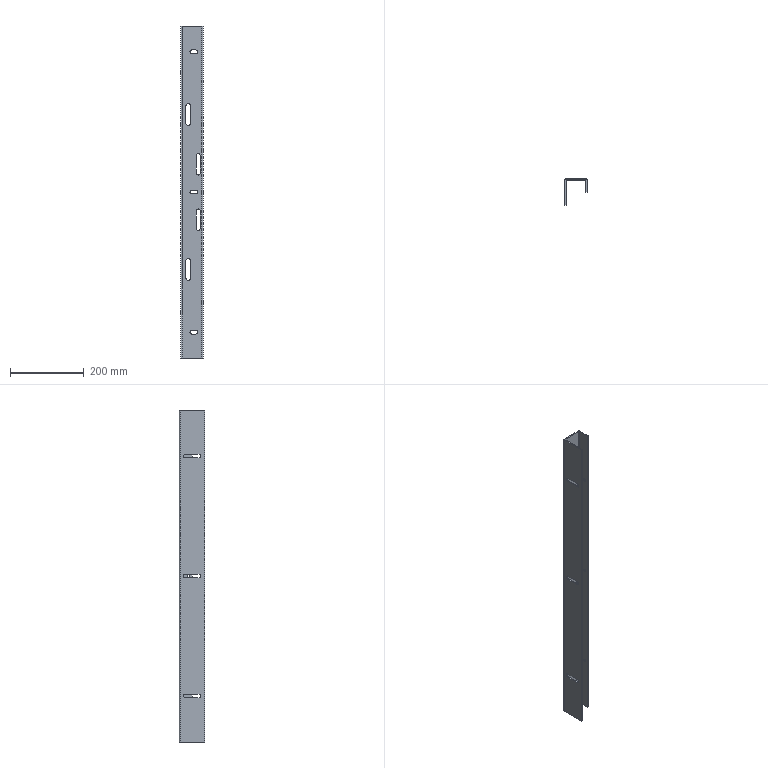Part | 1 solid | 71 faces | box 60 x 70 x 900 mm | volume 411225 mm3 | plane 38 | cylinder 33 | commonest cylinder face diameters 10 x19 7 x6 14 x4 0.4 x2 6.4 x2